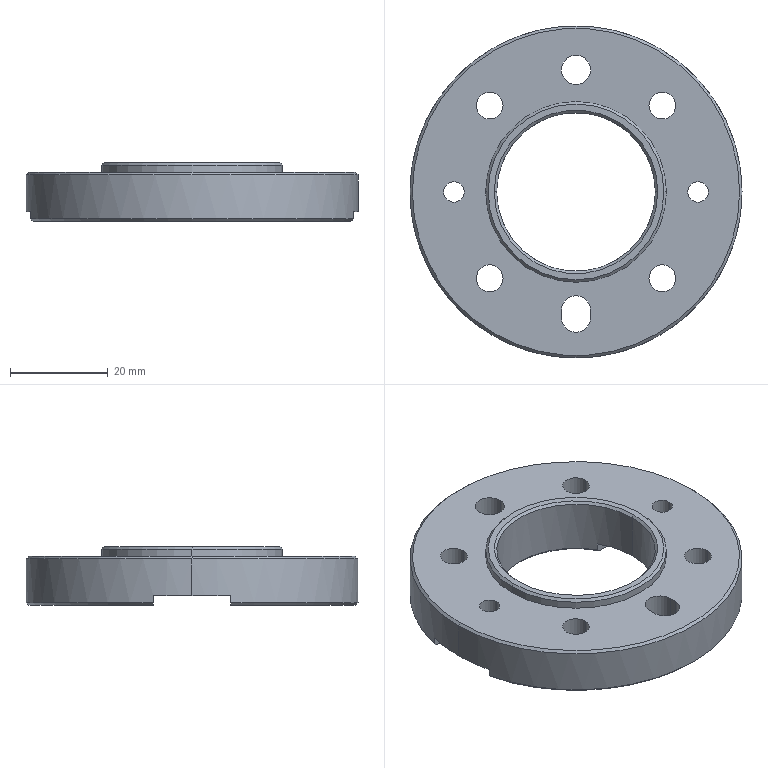Part | SolidWorks | features HoleWzd 4, Chamfer 1, ICE 1, Revolution 1 | 1 solid | 56 faces | box 68 x 68 x 12 mm | volume 24199 mm3 | cylinder 30 | plane 16 | cone 10 | commonest cylinder face diameters 5.5 x8 10 x8 4.2 x4 6 x4 32.5 x2 37 x2